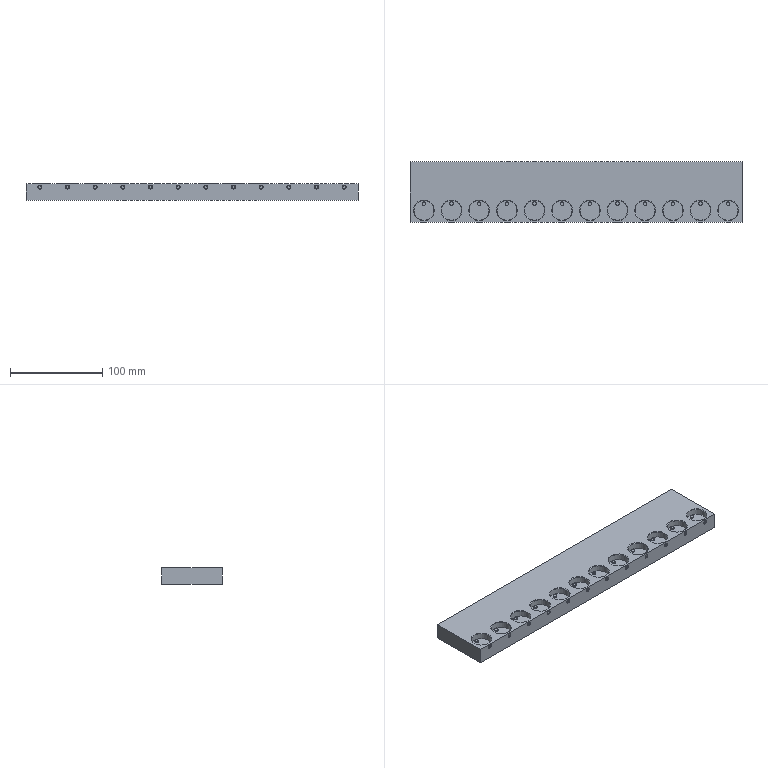NC program | NX | posted with a generic post | part box 360 x 66 x 17.6 mm
Whole program:
N10 G17 G21 G94 G90
(D1 , TOOL : 点钻D8-T4)
N12 T04 M6
N14 G54
N16 G17 G0 G90 X-15. Y3.5 B0. C0. S5000 M3
N18 G43 Z3. H4
N20 G94 G81 G99 Z-0.2 F250. R3.
N22 X-45.
N24 X-75.
N26 X-105.
N28 X-135.
N30 X-165.
N32 X-195.
N34 X-225.
N36 X-255.
N38 X-285.
N40 X-315.
N42 X-345.
N44 G80
N46 M5
(D2 , TOOL : 钻头3.3-T5)
N48 T05 M6
N50 G54
N52 G17 G0 G90 X-15. Y3.5 B0. C0. S1500 M3
N54 G43 Z3. H5
N56 G94 G83 G99 Z-6. F150. Q2. R3.
N58 X-45.
N60 X-75.
N62 X-105.
N64 X-135.
N66 X-165.
N68 X-195.
N70 X-225.
N72 X-255.
N74 X-285.
N76 X-315.
N78 X-345.
N80 G80
N82 M5
(D3 , TOOL : M4-T6)
N84 T06 M6
N86 G54
N88 G17 G0 G90 X-15. Y3.5 B0. C0. S300 M3
N90 G43 Z3. H6
N92 G94 G83 G99 Z-6. F1. Q2. R3.
N94 X-45.
N96 X-75.
N98 X-105.
N100 X-135.
N102 X-165.
N104 X-195.
N106 X-225.
N108 X-255.
N110 X-285.
N112 X-315.
N114 X-345.
N116 G80
N118 M5
N120 M2